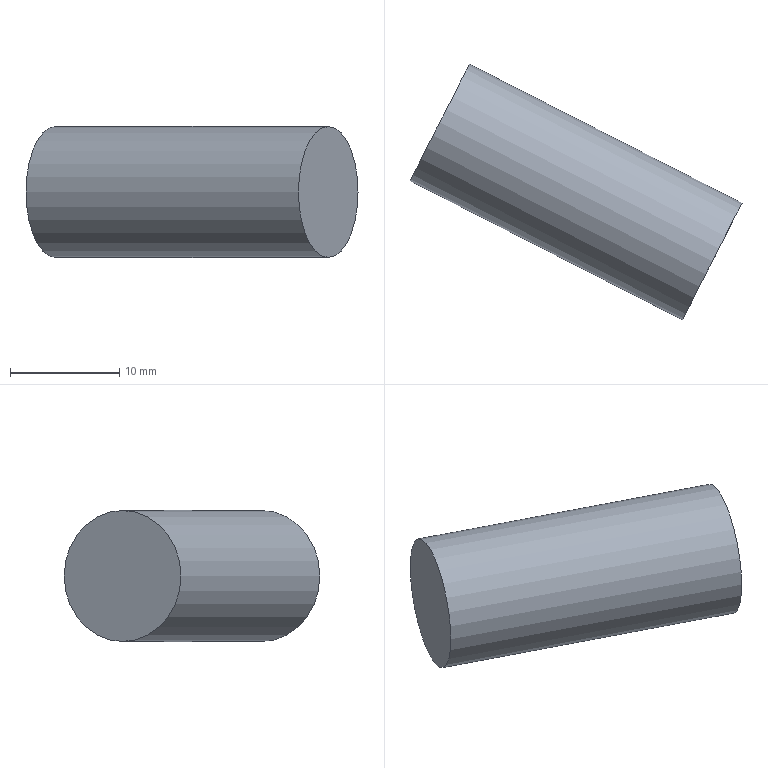Part | STEP file | gslz 2016.10.28-13_id1802_x_t | 1 solid | 3 faces | box 30.396 x 23.404 x 12 mm | volume 3167 mm3 | plane 2 | cylinder 1 | commonest cylinder face diameters 12 x1
STEP:
#1=CARTESIAN_POINT('',(0.,0.,0.));
#2=DIRECTION('',(0.,0.,1.));
#3=DIRECTION('',(1.,0.,0.));
#4=AXIS2_PLACEMENT_3D('',#1,#2,#3);
#5=CARTESIAN_POINT('',(1125.571,-35.997,-36.5));
#6=VERTEX_POINT('',#5);
#7=CARTESIAN_POINT('',(1122.847,-41.343,-36.5));
#8=DIRECTION('',(0.891,-0.454,0.));
#9=DIRECTION('',(0.454,0.891,0.));
#10=AXIS2_PLACEMENT_3D('',#7,#8,#9);
#11=CIRCLE('',#10,6.);
#12=CARTESIAN_POINT('',(1122.847,-41.343,-36.5));
#13=DIRECTION('',(-0.891,0.454,0.));
#14=DIRECTION('',(-0.454,-0.891,0.));
#15=AXIS2_PLACEMENT_3D('',#12,#13,#14);
#16=CYLINDRICAL_SURFACE('',#15,6.);
#17=CARTESIAN_POINT('',(9.425,0.));
#18=DIRECTION('',(-1.,0.));
#19=VECTOR('',#18,1.);
#20=LINE('',#17,#19);
#21=(GEOMETRIC_REPRESENTATION_CONTEXT(2)PARAMETRIC_REPRESENTATION_CONTEXT()REPRESENTATION_CONTEXT('',''));
#22=DEFINITIONAL_REPRESENTATION('',(#20),#21);
#23=PCURVE('',#16,#22);
#24=CARTESIAN_POINT('',(1122.847,-41.343,-36.5));
#25=DIRECTION('',(0.891,-0.454,0.));
#26=DIRECTION('',(0.454,0.891,0.));
#27=AXIS2_PLACEMENT_3D('',#24,#25,#26);
#28=PLANE('',#27);
#29=CARTESIAN_POINT('',(0.,0.));
#30=DIRECTION('',(1.,0.));
#31=AXIS2_PLACEMENT_2D('',#29,#30);
#32=CIRCLE('',#31,6.);
#33=(GEOMETRIC_REPRESENTATION_CONTEXT(2)PARAMETRIC_REPRESENTATION_CONTEXT()REPRESENTATION_CONTEXT('',''));
#34=DEFINITIONAL_REPRESENTATION('',(#32),#33);
#35=PCURVE('',#28,#34);
#36=SURFACE_CURVE('',#11,(#23,#35),.PCURVE_S1.);
#37=EDGE_CURVE('',#6,#6,#36,.T.);
#38=ORIENTED_EDGE('',*,*,#37,.F.);
#39=CARTESIAN_POINT('',(1100.623,-23.285,-36.5));
#40=VERTEX_POINT('',#39);
#41=CARTESIAN_POINT('',(1125.571,-35.997,-36.5));
#42=CARTESIAN_POINT('',(1100.623,-23.285,-36.5));
#43=B_SPLINE_CURVE_WITH_KNOTS('',1,(#41,#42),.UNSPECIFIED.,.F.,.F.,(2,2),(0.,28.),.PIECEWISE_BEZIER_KNOTS.);
#44=CARTESIAN_POINT('',(9.425,0.));
#45=DIRECTION('',(0.,1.));
#46=VECTOR('',#45,1.);
#47=LINE('',#44,#46);
#48=(GEOMETRIC_REPRESENTATION_CONTEXT(2)PARAMETRIC_REPRESENTATION_CONTEXT()REPRESENTATION_CONTEXT('',''));
#49=DEFINITIONAL_REPRESENTATION('',(#47),#48);
#50=PCURVE('',#16,#49);
#51=CARTESIAN_POINT('',(3.142,0.));
#52=DIRECTION('',(0.,1.));
#53=VECTOR('',#52,1.);
#54=LINE('',#51,#53);
#55=(GEOMETRIC_REPRESENTATION_CONTEXT(2)PARAMETRIC_REPRESENTATION_CONTEXT()REPRESENTATION_CONTEXT('',''));
#56=DEFINITIONAL_REPRESENTATION('',(#54),#55);
#57=PCURVE('',#16,#56);
#58=SEAM_CURVE('',#43,(#50,#57),.PCURVE_S1.);
#59=EDGE_CURVE('',#6,#40,#58,.T.);
#60=ORIENTED_EDGE('',*,*,#59,.T.);
#61=CARTESIAN_POINT('',(1097.899,-28.631,-36.5));
#62=DIRECTION('',(0.891,-0.454,0.));
#63=DIRECTION('',(0.454,0.891,0.));
#64=AXIS2_PLACEMENT_3D('',#61,#62,#63);
#65=CIRCLE('',#64,6.);
#66=CARTESIAN_POINT('',(9.425,28.));
#67=DIRECTION('',(-1.,0.));
#68=VECTOR('',#67,1.);
#69=LINE('',#66,#68);
#70=(GEOMETRIC_REPRESENTATION_CONTEXT(2)PARAMETRIC_REPRESENTATION_CONTEXT()REPRESENTATION_CONTEXT('',''));
#71=DEFINITIONAL_REPRESENTATION('',(#69),#70);
#72=PCURVE('',#16,#71);
#73=CARTESIAN_POINT('',(1097.899,-28.631,-36.5));
#74=DIRECTION('',(0.891,-0.454,0.));
#75=DIRECTION('',(0.454,0.891,0.));
#76=AXIS2_PLACEMENT_3D('',#73,#74,#75);
#77=PLANE('',#76);
#78=CARTESIAN_POINT('',(0.,0.));
#79=DIRECTION('',(1.,0.));
#80=AXIS2_PLACEMENT_2D('',#78,#79);
#81=CIRCLE('',#80,6.);
#82=(GEOMETRIC_REPRESENTATION_CONTEXT(2)PARAMETRIC_REPRESENTATION_CONTEXT()REPRESENTATION_CONTEXT('',''));
#83=DEFINITIONAL_REPRESENTATION('',(#81),#82);
#84=PCURVE('',#77,#83);
#85=SURFACE_CURVE('',#65,(#72,#84),.PCURVE_S1.);
#86=EDGE_CURVE('',#40,#40,#85,.T.);
#87=ORIENTED_EDGE('',*,*,#86,.T.);
#88=ORIENTED_EDGE('',*,*,#59,.F.);
#89=EDGE_LOOP('',(#38,#60,#87,#88));
#90=FACE_BOUND('',#89,.T.);
#91=ADVANCED_FACE('',(#90),#16,.T.);
#92=ORIENTED_EDGE('',*,*,#37,.T.);
#93=EDGE_LOOP('',(#92));
#94=FACE_BOUND('',#93,.T.);
#95=ADVANCED_FACE('',(#94),#28,.T.);
#96=ORIENTED_EDGE('',*,*,#86,.F.);
#97=EDGE_LOOP('',(#96));
#98=FACE_BOUND('',#97,.T.);
#99=ADVANCED_FACE('',(#98),#77,.F.);
#100=CLOSED_SHELL('',(#91,#95,#99));
#101=MANIFOLD_SOLID_BREP('',#100);
#102=(LENGTH_UNIT()NAMED_UNIT(*)SI_UNIT(.MILLI.,.METRE.));
#103=UNCERTAINTY_MEASURE_WITH_UNIT(LENGTH_MEASURE(0.00001),#102,'','');
#104=(NAMED_UNIT(*)PLANE_ANGLE_UNIT()SI_UNIT($,.RADIAN.));
#105=(NAMED_UNIT(*)SI_UNIT($,.STERADIAN.)SOLID_ANGLE_UNIT());
#106=(GEOMETRIC_REPRESENTATION_CONTEXT(3)GLOBAL_UNCERTAINTY_ASSIGNED_CONTEXT((#103))GLOBAL_UNIT_ASSIGNED_CONTEXT((#102,#104,#105))REPRESENTATION_CONTEXT('',''));
#107=ADVANCED_BREP_SHAPE_REPRESENTATION('',(#4,#101),#106);